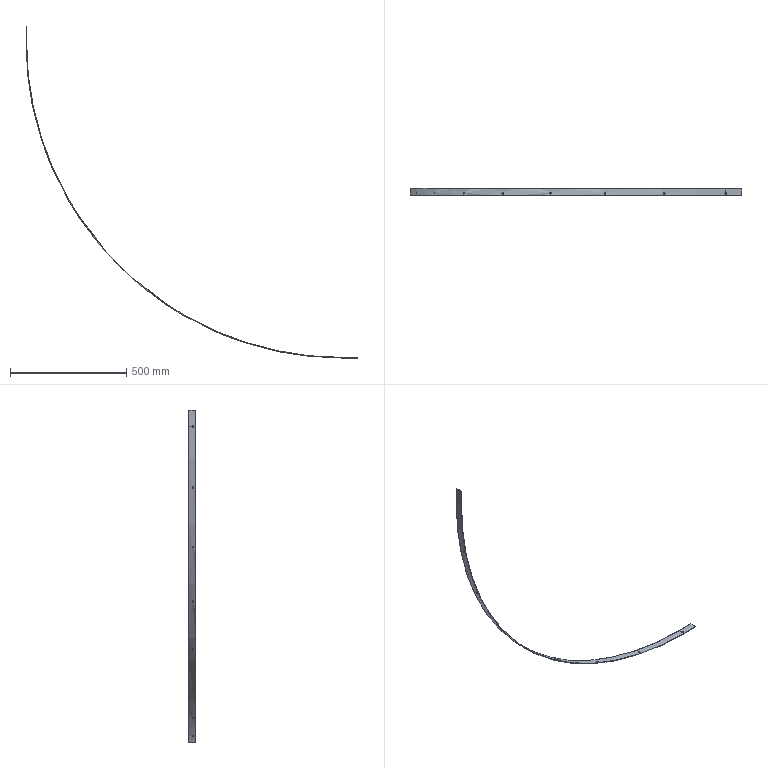Part | STEP file | covercurveroller-p1 | 1 solid | 35 faces | box 1431 x 30 x 1431 mm | volume 169835 mm3 | spline 14 | plane 8 | cone 7 | cylinder 6 | commonest cylinder face diameters 7 x4 2717 x1 2722 x1